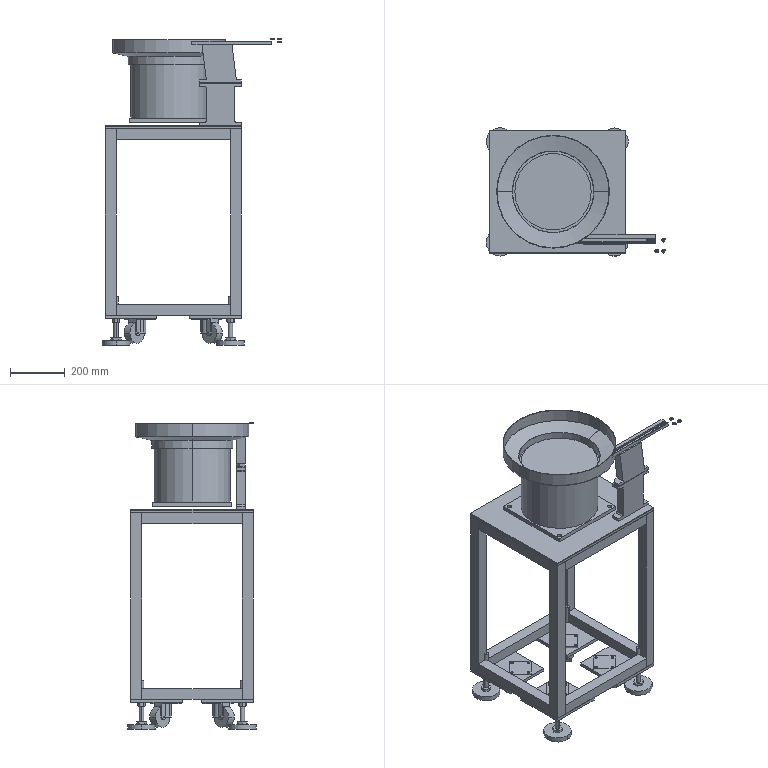Part | NX | 37 solids | 2893 faces | box 657.228 x 470 x 1125 mm | volume 33172115 mm3 | plane 1590 | cylinder 900 | cone 142 | spline 113 | torus 98 | sphere 50 | commonest cylinder face diameters 0.2 x264 1 x85 0.4 x60 8 x56 0.6 x40 6.75 x32